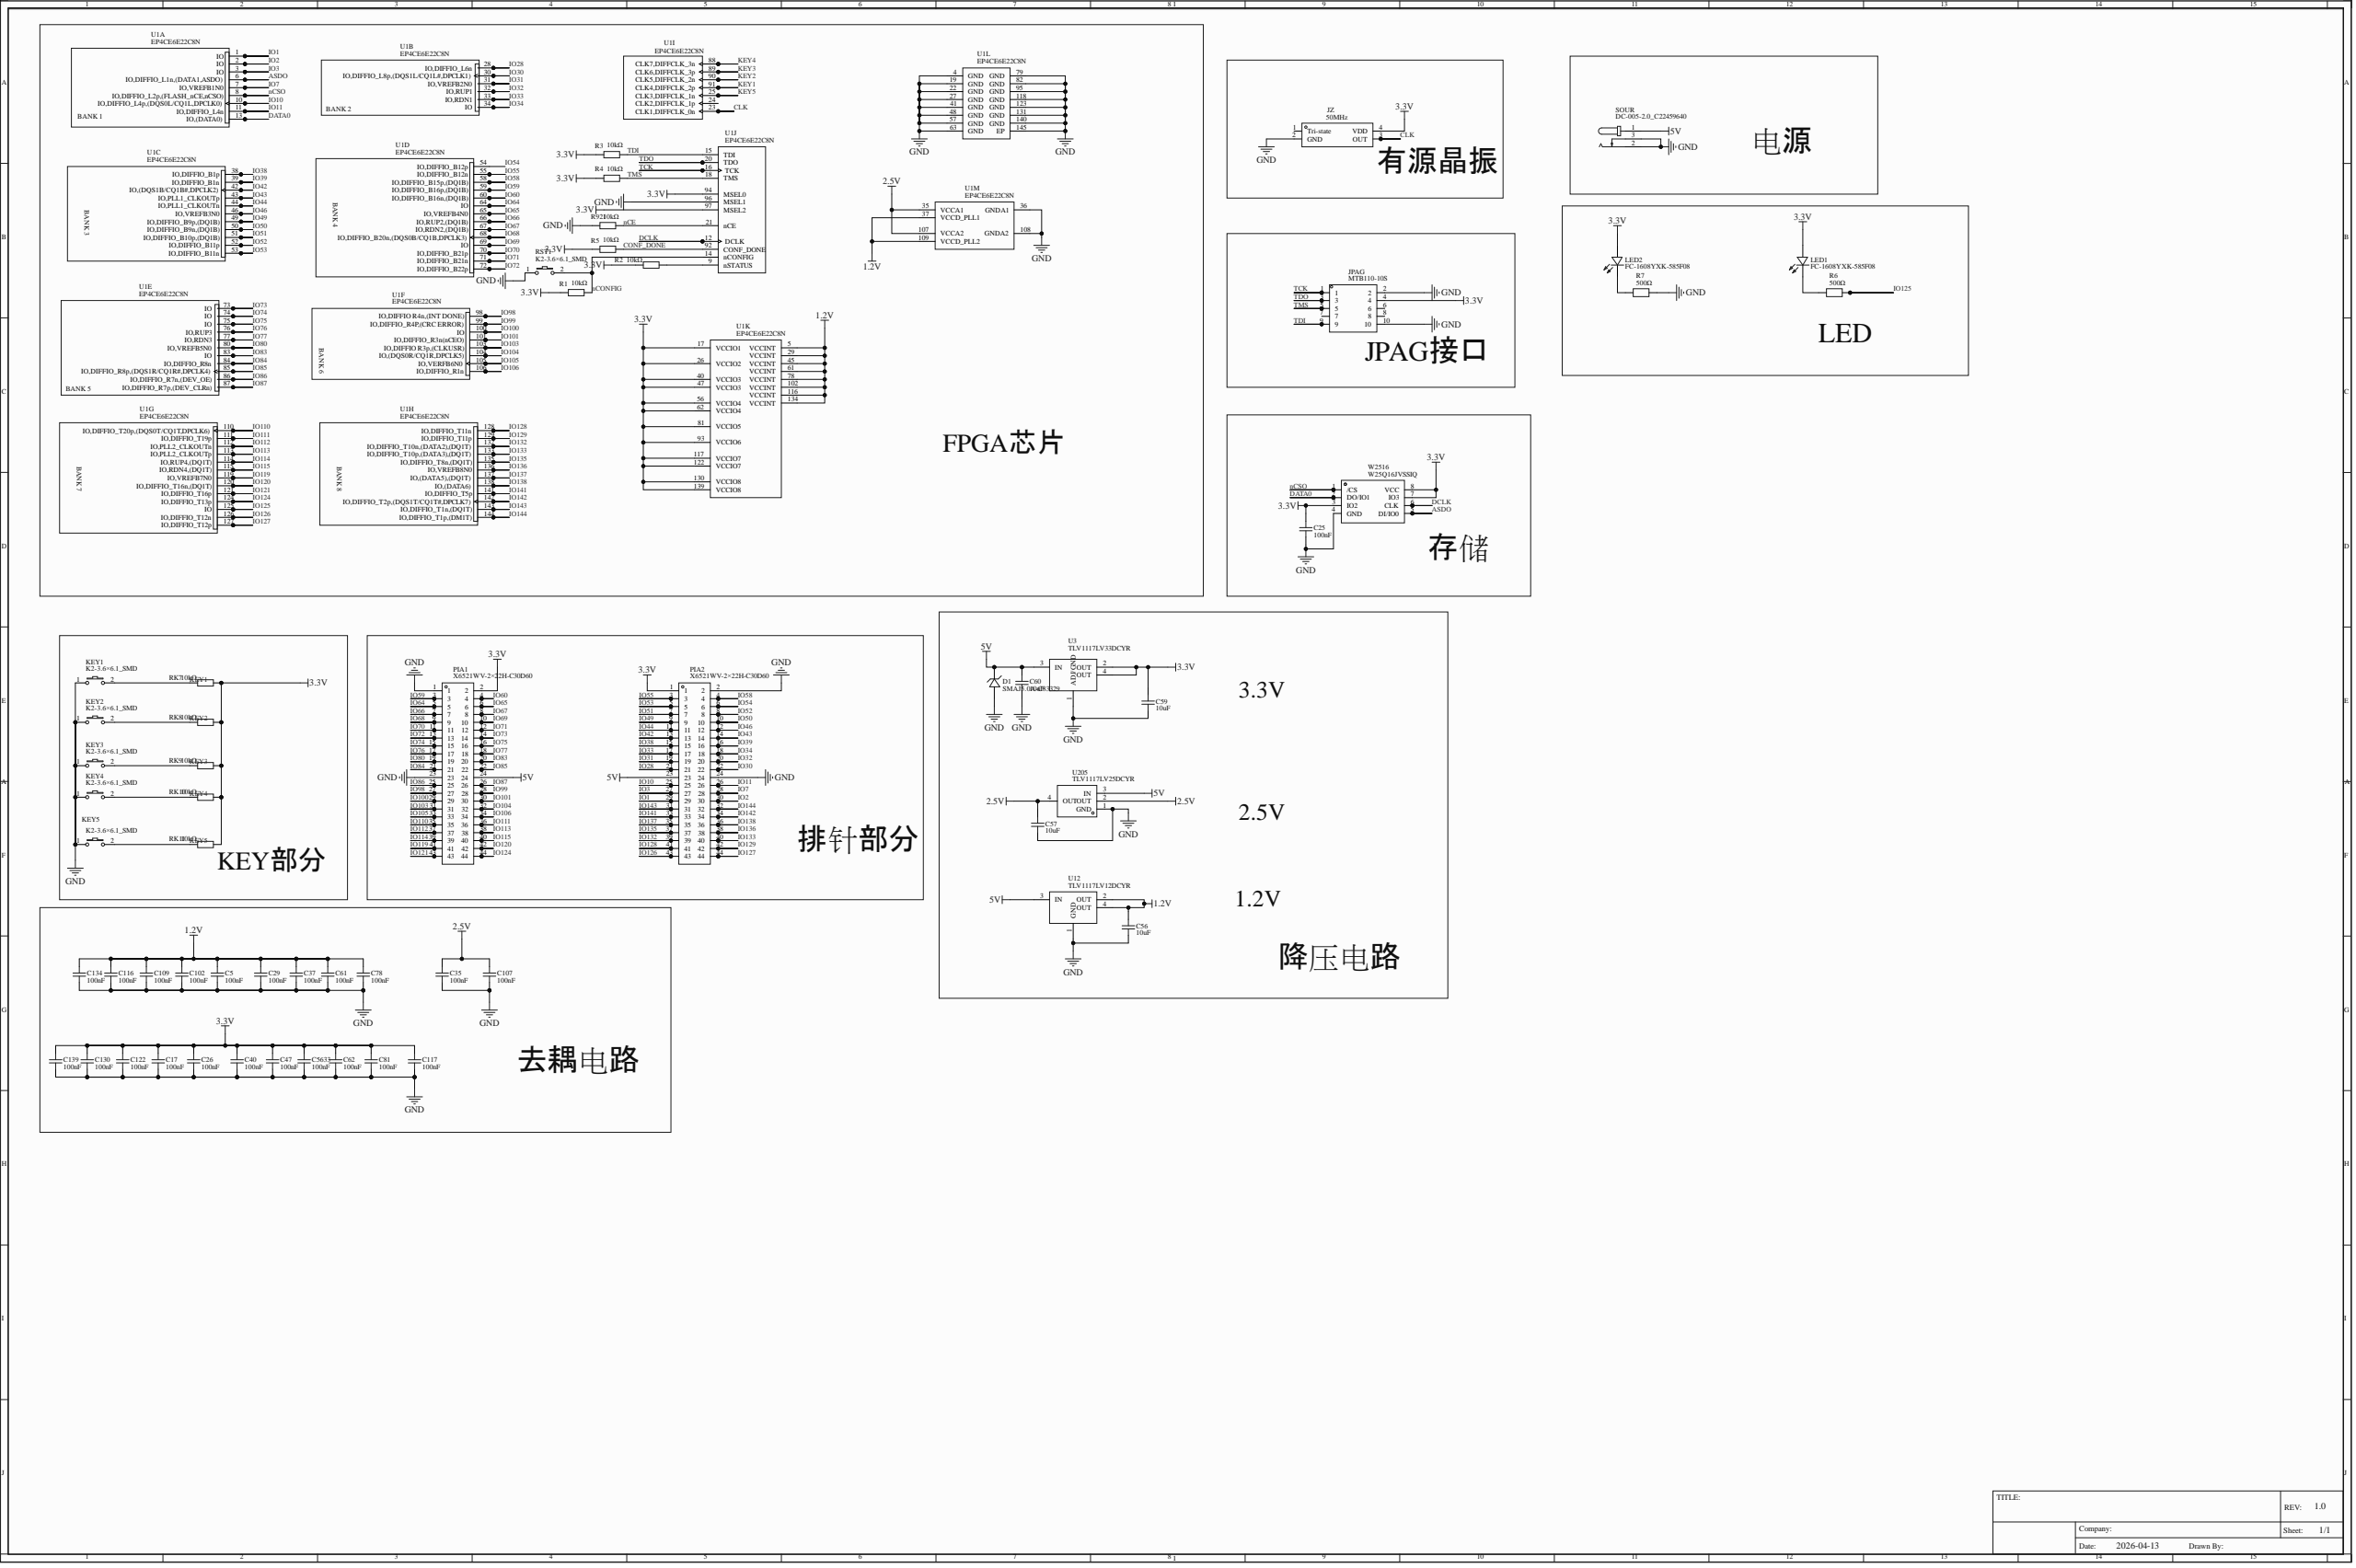Circuit board | Altium Designer | 59 parts | 106 nets
Bill of materials:
Comment,Description,Designator,Footprint,LibRef,Quantity
"100nF","","C5, C17, C25, C26, C29, C35, C37, C40, C47, C61, C62, C78, C81, C102, C107, C109, C116, C117, C122, C130, C134, C139, C5633","C0603","CGA0603X7R104K500JT","23"
"10uF","","C56, C57, C59, C60","C0603","CGA0603X5R106K100JT","4"
"SMAJ5.0A-C83329","","D1","SMA_L4.3-W2.6-LS5.2-RD","SMAJ5.0A","1"
"MTB110-10S","","JPAG","IDC-TH_MTB110-10S","MTB10-10S","1"
"50MHz","","JZ","OSC-SMD_4P-L5.0-W3.2-BL_7CZ-XXXXX","OT1EL89CJI-111YLC-50M","1"
"K2-3.6×6.1_SMD","","KEY1, KEY2, KEY3, KEY4, KEY5, RST1","KEY-SMD_2P-L6.2-W3.6-LS8.0","K2-1107ST-A4SW-06","6"
"FC-1608YXK-585F08","","LED1, LED2","LED0603-RD","NCD0603Y2","2"
"X6521WV-2×22H-C30D60","","PIA1, PIA2","HDR-TH_44P-2.54-V-M-R2-C22-S2.54","X6521WV-2x22H-C60D30","2"
"10kΩ","","R1, R2, R3, R4, R5, R921, RK7, RK8, RK9, RK10, RK11","R0402","RC0402FR-0710KL","11"
"500Ω","","R6, R7","R0805","ARG05BTC5000","2"
"DC-005-2.0_C22459640","","SOUR","DC-IN-TH_DC-005-2.0_C22459640","DC-005-2.0","1"
"EP4CE6E22C8N","","U1","PQFP-144_L20.0-W20.0-P0.50-LS22.0-BL-EP","EP4CE6E22C8N","1"
"TLV1117LV33DCYR","","U3","SOT-223_L6.7-W3.5-P2.30-BR","TLV1117LV33DCYR","1"
"TLV1117LV12DCYR","","U12","SOT-223-4_L6.5-W3.5-P2.30-LS7.0-BR","TLV1117LV12DCYR","1"
"TLV1117LV25DCYR","","U205","SOT-223-3_L6.5-W3.4-P2.30-LS7.0-BR","TLV1117LV25DCYR","1"
"W25Q16JVSSIQ","","W2516","SOIC-8_L5.3-W5.3-P1.27-LS8.0-BL","W25Q16JVSSIQ","1"
Netlist (Protel format):
[
C5
C0603
100nF



]
[
C17
C0603
100nF



]
[
C25
C0603
100nF



]
[
C26
C0603
100nF



]
[
C29
C0603
100nF



]
[
C35
C0603
100nF



]
[
C37
C0603
100nF



]
[
C40
C0603
100nF



]
[
C47
C0603
100nF



]
[
C56
C0603
10uF



]
[
C57
C0603
10uF



]
[
C59
C0603
10uF



]
[
C60
C0603
10uF



]
[
C61
C0603
100nF



]
[
C62
C0603
100nF



]
[
C78
C0603
100nF



]
[
C81
C0603
100nF



]
[
C102
C0603
100nF



]
[
C107
C0603
100nF



]
[
C109
C0603
100nF



]
[
C116
C0603
100nF



]
[
C117
C0603
100nF



]
[
C122
C0603
100nF



]
[
C130
C0603
100nF



]
[
C134
C0603
100nF



]
[
C139
C0603
100nF



]
[
C5633
C0603
100nF



]
[
D1
SMA_L4.3-W2.6-LS5.2-RD
SMAJ5.0A-C83329



]
[
JPAG
IDC-TH_MTB110-10S
MTB110-10S



]
[
JZ
OSC-SMD_4P-L5.0-W3.2-BL_7CZ-XXXXX
50MHz



]
[
KEY1
KEY-SMD_2P-L6.2-W3.6-LS8.0
K2-3.6×6.1_SMD



]
[
KEY2
KEY-SMD_2P-L6.2-W3.6-LS8.0
K2-3.6×6.1_SMD



]
[
KEY3
KEY-SMD_2P-L6.2-W3.6-LS8.0
K2-3.6×6.1_SMD



]
[
KEY4
KEY-SMD_2P-L6.2-W3.6-LS8.0
K2-3.6×6.1_SMD



]
[
KEY5
KEY-SMD_2P-L6.2-W3.6-LS8.0
K2-3.6×6.1_SMD



]
[
LED1
LED0603-RD
FC-1608YXK-585F08



]
[
LED2
LED0603-RD
FC-1608YXK-585F08



]
[
PIA1
HDR-TH_44P-2.54-V-M-R2-C22-S2.54
X6521WV-2×22H-C30D60



]
[
PIA2
HDR-TH_44P-2.54-V-M-R2-C22-S2.54
X6521WV-2×22H-C30D60



]
[
R1
R0402
10kΩ



]
[
R2
R0402
10kΩ



]
[
R3
R0402
10kΩ



]
[
R4
R0402
10kΩ



]
[
R5
R0402
10kΩ



]
[
R6
R0805
500Ω



]
[
R7
R0805
500Ω



]
[
R921
R0402
10kΩ



]
[
RK7
R0402
10kΩ



]
[
RK8
R0402
10kΩ



]
[
RK9
R0402
10kΩ



]
[
RK10
R0402
10kΩ



]
[
RK11
R0402
10kΩ



]
[
RST1
KEY-SMD_2P-L6.2-W3.6-LS8.0
K2-3.6×6.1_SMD



]
[
SOUR
DC-IN-TH_DC-005-2.0_C22459640
DC-005-2.0_C22459640



]
[
U1
PQFP-144_L20.0-W20.0-P0.50-LS22.0-BL-EP
EP4CE6E22C8N



]
[
U3
SOT-223_L6.7-W3.5-P2.30-BR
TLV1117LV33DCYR



]
[
U12
SOT-223-4_L6.5-W3.5-P2.30-LS7.0-BR
TLV1117LV12DCYR



]
[
U205
SOT-223-3_L6.5-W3.4-P2.30-LS7.0-BR
TLV1117LV25DCYR



]
[
W2516
SOIC-8_L5.3-W5.3-P1.27-LS8.0-BL
W25Q16JVSSIQ



]
(
TMS
JPAG-5
R4-2
U1-18
)
(
TDO
JPAG-3
U1-20
)
(
TDI
JPAG-9
R3-2
U1-15
)
(
TCK
JPAG-1
U1-16
)
(
NetR2_2
R2-2
U1-9
)
(
NetLED2_1
LED2-1
R7-1
)
(
NetLED1_1
LED1-1
R6-1
)
(
nCSO
U1-8
W2516-1
)
(
nCONFIG
R1-2
RST1-2
U1-14
)
(
nCE
R921-2
U1-21
)
(
KEY5
KEY5-2
RK11-1
U1-25
)
(
KEY4
KEY4-2
RK10-1
U1-88
)
(
KEY3
KEY3-2
RK9-1
U1-89
)
(
KEY2
KEY2-2
RK8-1
U1-90
)
(
KEY1
KEY1-2
RK7-1
U1-91
)
(
IO144
PIA2-32
U1-144
)
(
IO143
PIA2-31
U1-143
)
(
IO142
PIA2-34
U1-142
)
(
IO141
PIA2-33
U1-141
)
(
IO138
PIA2-36
U1-138
)
(
IO137
PIA2-35
U1-137
)
(
IO136
PIA2-38
U1-136
)
(
IO135
PIA2-37
U1-135
)
(
IO133
PIA2-40
U1-133
)
(
IO132
PIA2-39
U1-132
)
(
IO129
PIA2-42
U1-129
)
(
IO128
PIA2-41
U1-128
)
(
IO127
PIA2-44
U1-127
)
(
IO126
PIA2-43
U1-126
)
(
IO125
R6-2
U1-125
)
(
IO124
PIA1-44
U1-124
)
(
IO121
PIA1-43
U1-121
)
(
IO120
PIA1-42
U1-120
)
(
IO119
PIA1-41
U1-119
)
(
IO115
PIA1-40
U1-115
)
(
IO114
PIA1-39
U1-114
)
(
IO113
PIA1-38
U1-113
)
(
IO112
PIA1-37
U1-112
)
(
IO111
PIA1-36
U1-111
)
(
IO110
PIA1-35
U1-110
)
(
IO106
PIA1-34
U1-106
)
(
IO105
PIA1-33
U1-105
)
(
IO104
PIA1-32
U1-104
)
(
IO103
PIA1-31
U1-103
)
(
IO101
PIA1-30
U1-101
)
(
IO100
PIA1-29
U1-100
)
(
IO99
PIA1-28
U1-99
)
(
IO98
PIA1-27
U1-98
)
(
IO87
PIA1-26
U1-87
)
(
IO86
PIA1-25
U1-86
)
(
IO85
PIA1-22
U1-85
)
(
IO84
PIA1-21
U1-84
)
(
IO83
PIA1-20
U1-83
)
(
IO80
PIA1-19
U1-80
)
(
IO77
PIA1-18
U1-77
)
(
IO76
PIA1-17
U1-76
)
(
IO75
PIA1-16
U1-75
)
(
IO74
PIA1-15
U1-74
)
(
IO73
PIA1-14
U1-73
)
(
IO72
PIA1-13
U1-72
)
(
IO71
PIA1-12
U1-71
)
(
IO70
PIA1-11
U1-70
)
(
IO69
PIA1-10
U1-69
)
(
IO68
PIA1-9
U1-68
)
(
IO67
PIA1-8
U1-67
)
(
IO66
PIA1-7
U1-66
)
(
IO65
PIA1-6
U1-65
)
(
IO64
PIA1-5
U1-64
)
(
IO60
PIA1-4
U1-60
)
(
IO59
PIA1-3
U1-59
)
(
IO58
PIA2-4
U1-58
)
(
IO55
PIA2-3
U1-55
)
(
IO54
PIA2-6
U1-54
)
(
IO53
PIA2-5
U1-53
)
(
IO52
PIA2-8
U1-52
)
(
IO51
PIA2-7
U1-51
)
(
IO50
PIA2-10
U1-50
)
(
IO49
PIA2-9
U1-49
)
(
IO46
PIA2-12
U1-46
)
(
IO44
PIA2-11
U1-44
)
(
IO43
PIA2-14
U1-43
)
(
IO42
PIA2-13
U1-42
)
(
IO39
PIA2-16
U1-39
)
(
IO38
PIA2-15
U1-38
)
(
IO34
PIA2-18
U1-34
)
(
IO33
PIA2-17
U1-33
)
(
IO32
PIA2-20
U1-32
)
(
IO31
PIA2-19
U1-31
)
(
IO30
PIA2-22
U1-30
)
(
IO28
PIA2-21
U1-28
)
(
IO11
PIA2-26
U1-11
)
(
IO10
PIA2-25
U1-10
)
(
IO7
PIA2-28
U1-7
)
(
IO3
PIA2-27
U1-3
)
(
IO2
PIA2-30
U1-2
)
(
IO1
PIA2-29
U1-1
)
(
GND
C5-1
C17-1
C25-1
C26-1
C29-1
C35-1
C37-1
C40-1
C47-1
C56-1
C57-1
C59-1
C60-1
C61-1
C62-1
C78-1
C81-1
C102-1
C107-1
C109-1
C116-1
C117-1
C122-1
C130-1
C134-1
C139-1
C5633-1
D1-2
JPAG-2
JPAG-10
JZ-2
KEY1-1
KEY2-1
KEY3-1
KEY4-1
KEY5-1
PIA1-1
PIA1-23
PIA2-2
PIA2-24
R7-2
R921-1
RST1-1
SOUR-2
SOUR-3
U1-4
U1-19
U1-22
U1-27
U1-36
U1-41
U1-48
U1-57
U1-63
U1-79
U1-82
U1-95
U1-96
U1-108
U1-118
U1-123
U1-131
U1-140
U1-145
U3-1
U12-1
U205-1
W2516-4
)
(
DCLK
U1-12
W2516-6
)
(
DATA0
U1-13
W2516-2
)
(
CONF_DONE
R5-2
U1-92
)
(
CLK
JZ-3
U1-23
)
(
ASDO
U1-6
W2516-5
)
(
5V
C60-2
D1-1
PIA1-24
PIA2-23
SOUR-1
U3-3
U12-3
U205-3
)
(
3.3V
C17-2
C25-2
C26-2
C40-2
C47-2
C59-2
C62-2
C81-2
C117-2
C122-2
C130-2
C139-2
C5633-2
JPAG-4
JZ-4
LED1-2
LED2-2
PIA1-2
PIA2-1
R1-1
R2-1
R3-1
R4-1
R5-1
RK7-2
RK8-2
RK9-2
RK10-2
RK11-2
U1-17
U1-26
U1-40
U1-47
U1-56
U1-62
U1-81
U1-93
U1-94
U1-97
U1-117
U1-122
U1-130
U1-139
U3-2
U3-4
W2516-3
W2516-7
W2516-8
)
(
2.5V
C35-2
C57-2
C107-2
U1-35
U1-107
U205-2
U205-4
)
(
1.2V
C5-2
C29-2
C37-2
C56-2
C61-2
C78-2
C102-2
C109-2
C116-2
C134-2
U1-5
U1-29
U1-37
U1-45
U1-61
U1-78
U1-102
U1-109
U1-116
U1-134
U12-2
U12-4
)